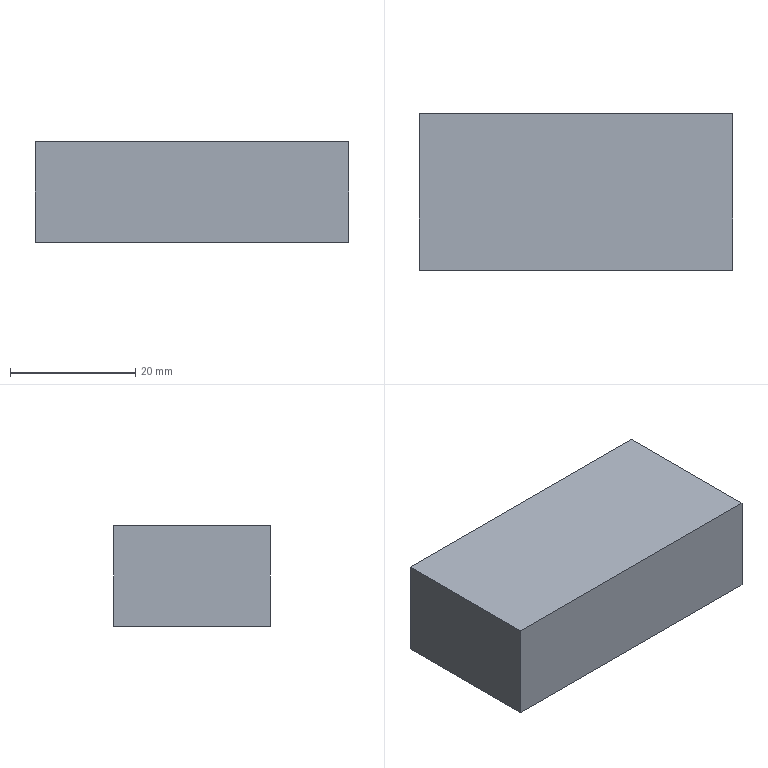Part | SolidWorks | features FlatPattern 1, SMBaseFlange 1, SheetMetal 1 | 1 solid | 6 faces | box 50 x 25 x 16 mm | volume 20000 mm3 | plane 6
STEP:
#1=CARTESIAN_POINT('',(0.,25.,0.));
#2=VERTEX_POINT('',#1);
#3=CARTESIAN_POINT('',(0.,0.,0.));
#4=VERTEX_POINT('',#3);
#5=CARTESIAN_POINT('',(0.,0.,0.));
#6=DIRECTION('',(0.,-1.,0.));
#7=VECTOR('',#6,1000.);
#8=LINE('',#5,#7);
#9=EDGE_CURVE('',#2,#4,#8,.T.);
#10=ORIENTED_EDGE('',*,*,#9,.F.);
#11=CARTESIAN_POINT('',(0.,25.,-16.));
#12=VERTEX_POINT('',#11);
#13=CARTESIAN_POINT('',(0.,25.,-16.));
#14=DIRECTION('',(0.,0.,1.));
#15=VECTOR('',#14,1000.);
#16=LINE('',#13,#15);
#17=EDGE_CURVE('',#12,#2,#16,.T.);
#18=ORIENTED_EDGE('',*,*,#17,.F.);
#19=CARTESIAN_POINT('',(0.,0.,-16.));
#20=VERTEX_POINT('',#19);
#21=CARTESIAN_POINT('',(0.,0.,-16.));
#22=DIRECTION('',(0.,-1.,0.));
#23=VECTOR('',#22,1000.);
#24=LINE('',#21,#23);
#25=EDGE_CURVE('',#12,#20,#24,.T.);
#26=ORIENTED_EDGE('',*,*,#25,.T.);
#27=CARTESIAN_POINT('',(0.,0.,-16.));
#28=DIRECTION('',(0.,0.,1.));
#29=VECTOR('',#28,1000.);
#30=LINE('',#27,#29);
#31=EDGE_CURVE('',#20,#4,#30,.T.);
#32=ORIENTED_EDGE('',*,*,#31,.T.);
#33=EDGE_LOOP('',(#10,#18,#26,#32));
#34=FACE_OUTER_BOUND('',#33,.T.);
#35=CARTESIAN_POINT('',(0.,0.,-16.));
#36=DIRECTION('',(-1.,0.,0.));
#37=DIRECTION('',(0.,0.,1.));
#38=AXIS2_PLACEMENT_3D('',#35,#36,#37);
#39=PLANE('',#38);
#40=ADVANCED_FACE('',(#34),#39,.T.);
#41=CARTESIAN_POINT('',(50.,25.,0.));
#42=VERTEX_POINT('',#41);
#43=CARTESIAN_POINT('',(0.,25.,0.));
#44=DIRECTION('',(-1.,0.,0.));
#45=VECTOR('',#44,1000.);
#46=LINE('',#43,#45);
#47=EDGE_CURVE('',#42,#2,#46,.T.);
#48=ORIENTED_EDGE('',*,*,#47,.F.);
#49=CARTESIAN_POINT('',(50.,25.,-16.));
#50=VERTEX_POINT('',#49);
#51=CARTESIAN_POINT('',(50.,25.,-16.));
#52=DIRECTION('',(0.,0.,1.));
#53=VECTOR('',#52,1000.);
#54=LINE('',#51,#53);
#55=EDGE_CURVE('',#50,#42,#54,.T.);
#56=ORIENTED_EDGE('',*,*,#55,.F.);
#57=CARTESIAN_POINT('',(0.,25.,-16.));
#58=DIRECTION('',(-1.,0.,0.));
#59=VECTOR('',#58,1000.);
#60=LINE('',#57,#59);
#61=EDGE_CURVE('',#50,#12,#60,.T.);
#62=ORIENTED_EDGE('',*,*,#61,.T.);
#63=ORIENTED_EDGE('',*,*,#17,.T.);
#64=EDGE_LOOP('',(#48,#56,#62,#63));
#65=FACE_OUTER_BOUND('',#64,.T.);
#66=CARTESIAN_POINT('',(0.,25.,-16.));
#67=DIRECTION('',(0.,1.,0.));
#68=DIRECTION('',(0.,0.,1.));
#69=AXIS2_PLACEMENT_3D('',#66,#67,#68);
#70=PLANE('',#69);
#71=ADVANCED_FACE('',(#65),#70,.T.);
#72=CARTESIAN_POINT('',(50.,0.,0.));
#73=VERTEX_POINT('',#72);
#74=CARTESIAN_POINT('',(50.,0.,0.));
#75=DIRECTION('',(0.,1.,0.));
#76=VECTOR('',#75,1000.);
#77=LINE('',#74,#76);
#78=EDGE_CURVE('',#73,#42,#77,.T.);
#79=ORIENTED_EDGE('',*,*,#78,.F.);
#80=CARTESIAN_POINT('',(50.,0.,-16.));
#81=VERTEX_POINT('',#80);
#82=CARTESIAN_POINT('',(50.,0.,-16.));
#83=DIRECTION('',(0.,0.,1.));
#84=VECTOR('',#83,1000.);
#85=LINE('',#82,#84);
#86=EDGE_CURVE('',#81,#73,#85,.T.);
#87=ORIENTED_EDGE('',*,*,#86,.F.);
#88=CARTESIAN_POINT('',(50.,0.,-16.));
#89=DIRECTION('',(0.,1.,0.));
#90=VECTOR('',#89,1000.);
#91=LINE('',#88,#90);
#92=EDGE_CURVE('',#81,#50,#91,.T.);
#93=ORIENTED_EDGE('',*,*,#92,.T.);
#94=ORIENTED_EDGE('',*,*,#55,.T.);
#95=EDGE_LOOP('',(#79,#87,#93,#94));
#96=FACE_OUTER_BOUND('',#95,.T.);
#97=CARTESIAN_POINT('',(50.,0.,-16.));
#98=DIRECTION('',(1.,0.,0.));
#99=DIRECTION('',(0.,0.,-1.));
#100=AXIS2_PLACEMENT_3D('',#97,#98,#99);
#101=PLANE('',#100);
#102=ADVANCED_FACE('',(#96),#101,.T.);
#103=CARTESIAN_POINT('',(0.,0.,0.));
#104=DIRECTION('',(1.,0.,0.));
#105=VECTOR('',#104,1000.);
#106=LINE('',#103,#105);
#107=EDGE_CURVE('',#4,#73,#106,.T.);
#108=ORIENTED_EDGE('',*,*,#107,.F.);
#109=ORIENTED_EDGE('',*,*,#31,.F.);
#110=CARTESIAN_POINT('',(0.,0.,-16.));
#111=DIRECTION('',(1.,0.,0.));
#112=VECTOR('',#111,1000.);
#113=LINE('',#110,#112);
#114=EDGE_CURVE('',#20,#81,#113,.T.);
#115=ORIENTED_EDGE('',*,*,#114,.T.);
#116=ORIENTED_EDGE('',*,*,#86,.T.);
#117=EDGE_LOOP('',(#108,#109,#115,#116));
#118=FACE_OUTER_BOUND('',#117,.T.);
#119=CARTESIAN_POINT('',(0.,0.,-16.));
#120=DIRECTION('',(0.,-1.,0.));
#121=DIRECTION('',(0.,0.,-1.));
#122=AXIS2_PLACEMENT_3D('',#119,#120,#121);
#123=PLANE('',#122);
#124=ADVANCED_FACE('',(#118),#123,.T.);
#125=ORIENTED_EDGE('',*,*,#25,.F.);
#126=ORIENTED_EDGE('',*,*,#61,.F.);
#127=ORIENTED_EDGE('',*,*,#92,.F.);
#128=ORIENTED_EDGE('',*,*,#114,.F.);
#129=EDGE_LOOP('',(#125,#126,#127,#128));
#130=FACE_OUTER_BOUND('',#129,.T.);
#131=CARTESIAN_POINT('',(0.,0.,-16.));
#132=DIRECTION('',(0.,0.,-1.));
#133=DIRECTION('',(-1.,0.,0.));
#134=AXIS2_PLACEMENT_3D('',#131,#132,#133);
#135=PLANE('',#134);
#136=ADVANCED_FACE('',(#130),#135,.T.);
#137=ORIENTED_EDGE('',*,*,#9,.T.);
#138=ORIENTED_EDGE('',*,*,#107,.T.);
#139=ORIENTED_EDGE('',*,*,#78,.T.);
#140=ORIENTED_EDGE('',*,*,#47,.T.);
#141=EDGE_LOOP('',(#137,#138,#139,#140));
#142=FACE_OUTER_BOUND('',#141,.T.);
#143=CARTESIAN_POINT('',(0.,0.,0.));
#144=DIRECTION('',(0.,0.,-1.));
#145=DIRECTION('',(-1.,0.,0.));
#146=AXIS2_PLACEMENT_3D('',#143,#144,#145);
#147=PLANE('',#146);
#148=ADVANCED_FACE('',(#142),#147,.F.);
#149=CLOSED_SHELL('',(#40,#71,#102,#124,#136,#148));
#150=MANIFOLD_SOLID_BREP('',#149);
#151=CARTESIAN_POINT('',(0.,0.,0.));
#152=DIRECTION('',(0.,0.,1.));
#153=DIRECTION('',(1.,0.,0.));
#154=AXIS2_PLACEMENT_3D('',#151,#152,#153);
#155=(LENGTH_UNIT()NAMED_UNIT(*)SI_UNIT(.MILLI.,.METRE.));
#156=UNCERTAINTY_MEASURE_WITH_UNIT(LENGTH_MEASURE(0.00001),#155,'','');
#157=(NAMED_UNIT(*)PLANE_ANGLE_UNIT()SI_UNIT($,.RADIAN.));
#158=(NAMED_UNIT(*)SI_UNIT($,.STERADIAN.)SOLID_ANGLE_UNIT());
#159=(GEOMETRIC_REPRESENTATION_CONTEXT(3)GLOBAL_UNCERTAINTY_ASSIGNED_CONTEXT((#156))GLOBAL_UNIT_ASSIGNED_CONTEXT((#155,#157,#158))REPRESENTATION_CONTEXT('',''));
#160=ADVANCED_BREP_SHAPE_REPRESENTATION('',(#150,#154),#159);